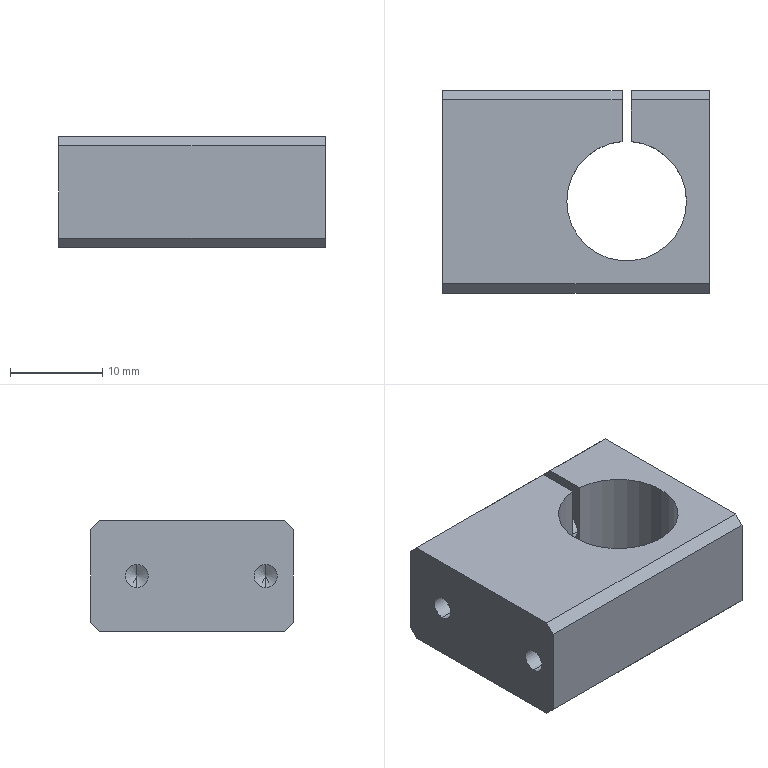NC program | NX | posted with a generic post | part box 29 x 22 x 12 mm
Whole program:
N10 G17 G21 G94 G90
(FLOOR_WALL_COPY , TOOL : D63)
N12 T03 M6
N14 G54
N16 G17 G0 G90 X-48.999 Y0. B0. C0. S6500 M3
N18 G43 Z30. H3
N20 Z3.
N22 G94 G1 Z0. F1250.
N24 X-45.999
N26 X45.999
N28 X48.999
N30 Z3.
N32 G0 Z30.
N34 M5
(ADAPTIVE_MILLING_COPY , TOOL : D10)
N36 T04 M6
N38 G54
N40 G17 G0 G90 X-27.209 Y-0.062 B0. C0. S9500 M3
N42 G43 Z30. H4
N44 Z-11.
N46 G94 G1 Z-12. F1000.
N48 X-26.429 Y-0.341 F3500.
N50 X-25.64 Y-0.597
N52 G3 X-24.562 Y-0.062 R1.017
N54 X-23.801 Y3.002 R8.28
N56 X-23.518 Y12.994 R113.543
N58 G2 X-21.123 Y17.326 R5.64
N60 X-15.583 Y19.467 R12.233
N62 X-7.48 Y19.952 R57.453
N64 G1 X-6.48 Y19.962
N66 X-5.105 Y19.972
N68 X-3.605 Y19.979
N70 X-1.355 Y19.984
N72 X2.27 Y19.987
N74 X13.77 Y19.988
N76 G2 X17.266 Y19.918 R28.437
N78 X21.271 Y16.958 R6.211
N80 X23.095 Y11.163 R14.093
N82 X23.469 Y2.3 R82.244
N84 G1 X23.477 Y0.8
N86 X23.482 Y-1.2
N88 X23.486 Y-4.2
N90 X23.488 Y-10.7
N92 Y-13.075
N94 X23.484 Y-13.2
N96 X23.477 Y-13.325
N98 X23.465 Y-13.449
N100 G2 X20.623 Y-17.666 R6.024
N102 X14.856 Y-19.569 R13.682
N104 X5.496 Y-19.97 R81.258
N106 G1 X3.996 Y-19.977
N108 X1.996 Y-19.983
N110 X-1.129 Y-19.986
N112 X-8.504 Y-19.988
N114 X-16.504
N116 X-16.629 Y-19.986
N118 G2 X-20.831 Y-17.582 R5.703
N120 X-22.984 Y-11.917 R12.284
N122 X-23.38 Y-2.189 R53.839
N124 G3 X-22.54 Y10.525 R109.542
N126 G2 X-18.854 Y16.329 R7.745
N128 X-12.508 Y18.463 R15.474
N130 X-3.152 Y18.946 R75.766
N132 X14.097 Y18.948 R852.674
N134 X19.875 Y15.226 R7.709
N136 X21.995 Y8.743 R15.825
N138 X22.446 Y-0.365 R77.137
N140 X22.446 Y-10.614 R486.261
N142 X18.711 Y-16.384 R7.719
N144 X12.226 Y-18.496 R15.829
N146 X2.868 Y-18.948 R79.444
N148 X-14.131 Y-18.945 R801.145
N150 X-19.958 Y-15.088 R7.756
N152 X-22.001 Y-8.707 R16.07
N154 X-22.091 Y-0.476 R36.073
N156 G3 X-21.577 Y8.508 R564.861
N158 G2 X-18.319 Y14.411 R8.811
N160 X-15.772 Y16.083 R6.237
N162 X-8.345 Y17.662 R24.178
N164 X5.398 Y17.96 R200.439
N166 X12.022 Y17.911 R121.987
N168 X17.655 Y15.015 R8.536
N170 X19.218 Y13.067 R5.093
N172 X21.095 Y5.592 R21.508
N174 X21.416 Y-8.398 R142.323
N176 X18.524 Y-14.143 R8.522
N178 X16.567 Y-15.717 R5.089
N180 X9.092 Y-17.594 R21.488
N182 X-2.524 Y-17.952 R138.09
N184 X-11.898 Y-17.922 R256.166
N186 X-17.646 Y-15.022 R8.547
N188 X-19.217 Y-13.067 R5.088
N190 X-21.073 Y-4.334 R20.582
N192 X-20.627 Y6.653 R173.549
N194 X-19.673 Y10.006 R12.485
N196 X-19.448 Y12.397 R13.286
N198 X-18.309 Y14.424 R5.576
N200 G1 X-18.086 Y14.684
N202 X-17.13 Y15.418
N204 X-17.011 Y15.487
N206 G2 X-14.215 Y16.158 R6.147
N208 X-5.364 Y16.783 R256.615
N210 X9.759 Y16.913 R318.962
N212 X13.161 Y16.155 R13.912
N214 X15.897 Y15.948 R11.759
N216 X17.725 Y14.961 R5.27
N218 G3 X18.442 Y16.933 R-1.1
N220 G1 X-14.418 Y18.349
N222 G3 X-14.465 Y16.15 R-1.1
N224 G1 X13.285
N226 G2 X15.897 Y15.948 R10.833
N228 X18.987 Y13.511 R5.458
N230 X19.658 Y10.715 R6.147
N232 X20.301 Y1.364 R245.433
N234 X20.364 Y-6.633 R93.463
N236 X19.669 Y-9.541 R11.27
N238 X19.448 Y-12.397 R14.397
N240 X18.461 Y-14.225 R5.27
N242 G3 X20.432 Y-14.955 R-1.1
N244 G1 X21.848 Y10.905
N246 G3 X19.65 Y10.965 R-1.1
N248 G1 Y-9.785
N250 G2 X19.448 Y-12.397 R10.833
N252 X17.011 Y-15.487 R5.458
N254 X14.09 Y-16.163 R6.279
N256 X-4.51 Y-16.941 R180.819
N258 X-10.133 Y-16.882 R83.077
N260 X-13.161 Y-16.154 R14.918
N262 X-15.897 Y-15.948 R11.699
N264 X-17.725 Y-14.961 R5.27
N266 G3 X-18.442 Y-16.933 R-1.1
N268 G1 X14.418 Y-18.349
N270 G3 X14.465 Y-16.15 R-1.1
N272 G1 X-13.285
N274 G2 X-15.897 Y-15.948 R10.833
N276 X-18.987 Y-13.511 R5.458
N278 X-19.654 Y-10.715 R6.07
N280 X-19.65 Y5.096 R93.047
N282 G1 Y10.221
N284 G3 X-20.752 Y11.319 R1.1
N286 X-21.85 Y10.221 R1.1
N288 G1 Y-10.84
N290 G3 X-20.748 Y-11.938 R1.1
N292 X-19.65 Y-10.84 R1.1
N294 G1 Y5.16
N296 G3 X-20.516 Y6.16 R1.016
N298 G1 X-22.11 Y6.389
N300 Z-9.
N302 G0 Z30.
(HOLE_MILLING , TOOL : D10)
N304 X5.5 Y-1.
N306 Z0.5
N308 G3 X6.2 Y-1.7 R0.7 F2000.
N310 X6.9 Y-1. R0.7
N312 X6.9 Y-1. Z-0.5 I-1.4 J0.
N314 X6.9 Y-1. Z-1.5 I-1.4 J0.
N316 X6.9 Y-1. Z-2.5 I-1.4 J0.
N318 X6.9 Y-1. Z-3.5 I-1.4 J0.
N320 X6.9 Y-1. Z-4.5 I-1.4 J0.
N322 X6.9 Y-1. Z-5.5 I-1.4 J0.
N324 X6.9 Y-1. Z-6.5 I-1.4 J0.
N326 X6.9 Y-1. Z-7.5 I-1.4 J0.
N328 X6.9 Y-1. Z-8.5 I-1.4 J0.
N330 X6.9 Y-1. Z-9.5 I-1.4 J0.
N332 X6.9 Y-1. Z-10.5 I-1.4 J0.
N334 X6.9 Y-1. Z-11.5 I-1.4 J0.
N336 X4.1 Y-1. Z-12. I-1.4 J0.
N338 X5.5 Y-2.4 R1.4
N340 X4.1 Y-1. R-1.4
N342 X4.8 Y-1.7 R0.7
N344 X5.5 Y-1. R0.7
N346 G0 Z30.
N348 M5
(ZLEVEL_PROFILE_1_COPY , TOOL : D6JING)
N350 T16 M6
N352 G54
N354 G17 G0 G90 X-15.158 Y14.539 B0. C0. S9500 M3
N356 G43 Z30. H16
N358 Z-11.
N360 G94 G1 Z-12. F1000.
N362 X-15.02 Y14.3
N364 G3 X-14.5 Y14. R0.6
N366 G1 X5.
N368 G2 X5.5 Y13.958 R3.
N370 X6. Y14. R3.
N372 G1 X14.5
N374 G2 X17.5 Y11. R3.
N376 G1 Y-11.
N378 G2 X14.5 Y-14. R3.
N380 G1 X-14.5
N382 G2 X-17.5 Y-11. R3.
N384 G1 Y11.
N386 G2 X-14.5 Y14. R3.
N388 G3 X-13.98 Y14.3 R0.6
N390 G1 X-13.807 Y14.6
N392 Z-11.
N394 G0 Z30.
N396 M5
(11_COPY_COPY , TOOL : D6A45)
N398 T01 M6
N400 G54
N402 G17 G0 G90 X6.863 Y2.592 B0. C0. S9500 M3
N404 G43 Z30. H1
N406 Z1.5
N408 G94 G1 Z-1.5 F1000.
N410 X6.374 Y3.676
N412 G3 X5.887 Y4.027 R0.6
N414 G1 X5.836 Y4.032
N416 X5.512 Y4.109
N418 X5.502 Y4.113
N420 G2 X5.113 Y4.027 R1.504
N422 G3 X5.887 Y4.027 R-5.041
N424 X5.346 Y3.767 R0.6
N426 G1 X4.646 Y2.745
N428 Z1.5
N430 G0 Z30.
N432 X15.441 Y-12.487
N434 Z1.5
N436 G1 Z-1.5
N438 X15.02 Y-11.759
N440 G3 X14.501 Y-11.459 R0.6
N442 G1 X-14.501
N444 G2 X-15.959 Y-10.001 R1.458
N446 G1 Y10.001
N448 G2 X-14.501 Y11.459 R1.458
N450 G1 X5.001
N452 G2 X5.498 Y11.368 R1.42
N454 X5.999 Y11.459 R1.472
N456 G1 X14.501
N458 G2 X15.959 Y10.001 R1.458
N460 G1 Y-10.001
N462 G2 X14.501 Y-11.459 R1.458
N464 G3 X13.981 Y-11.759 R0.6
N466 G1 X13.461 Y-12.659
N468 Z1.5
N470 G0 Z30.
N472 M5
(CUTTERCOMP16 , TOOL : D6JING)
N474 T16 M6
N476 G54
N478 G17 G0 G90 X5.5 Y-1. B0. C0. S9500 M3
N480 G43 Z30. H16
N482 Z0.5
N484 G41 G94 G1 X5.523 Y-1.399 F1000. D16
N486 G3 X8.95 Y-1. R1.737
N488 X8.95 Y-1. Z-2.5 I-3.45 J0.
N490 X8.95 Y-1. Z-5.5 I-3.45 J0.
N492 X8.95 Y-1. Z-8.5 I-3.45 J0.
N494 X8.95 Y-1. Z-11.5 I-3.45 J0.
N496 X7.225 Y1.988 Z-12. R3.45
N498 X2.512 Y0.725 R3.45
N500 X7.225 Y1.988 R-3.45
N502 X5.166 Y-0.78 R1.737
N504 G40
N506 G1 X5.5 Y-1.
N508 G0 Z30.
N510 M5
N512 M2